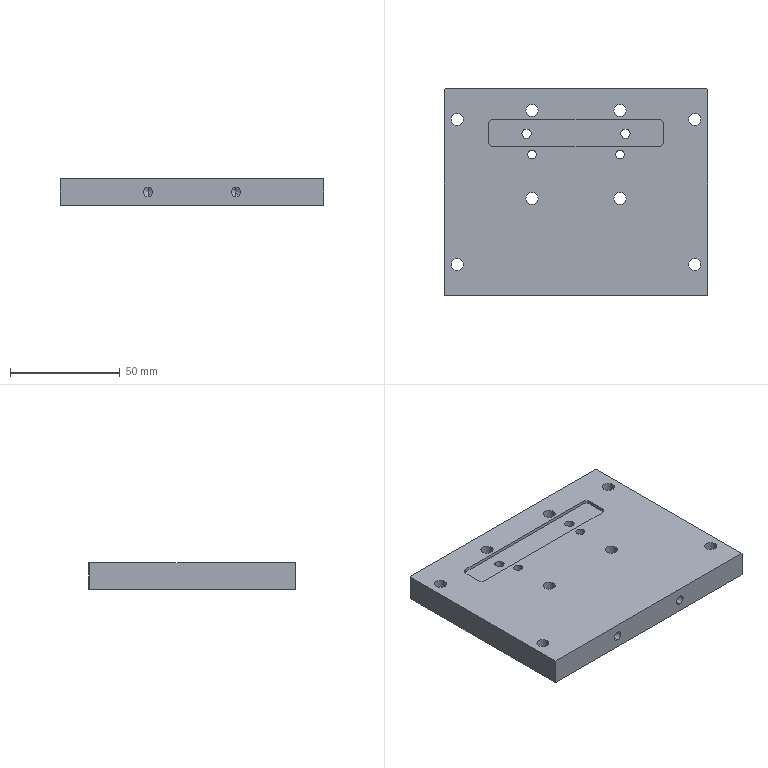Part | STEP file | 2044 Support plate 2 | 1 solid | 61 faces | box 120 x 94 x 12 mm | volume 129518 mm3 | cylinder 40 | plane 17 | cone 4 | commonest cylinder face diameters 5.5 x16 4.2 x8 9.5 x8 4 x4 5 x4